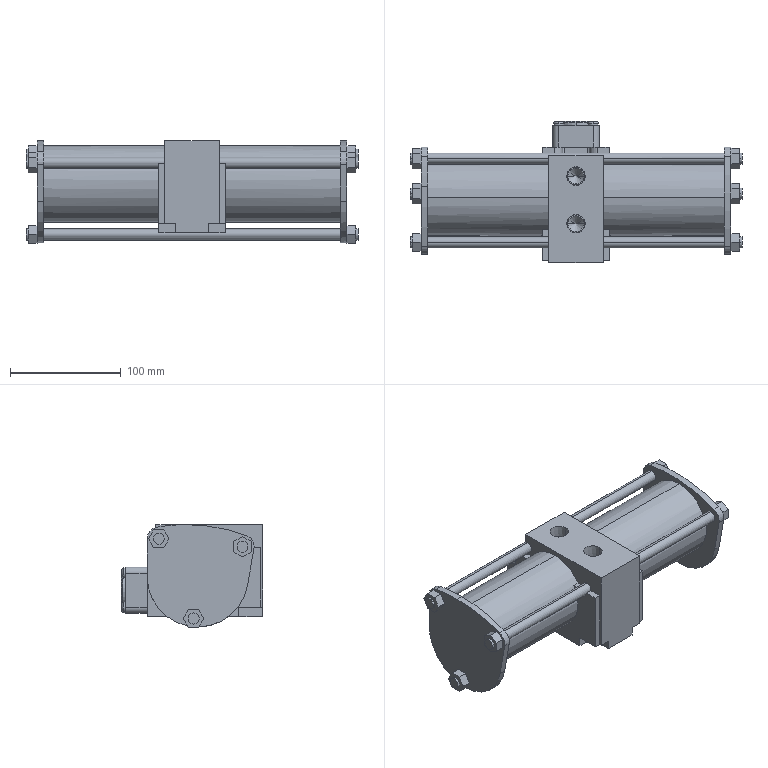Part | STEP file | VBA22A-03GN_VBA20A Body | 1 solid | 199 faces | box 300 x 127.5 x 92.8 mm | volume 1446394 mm3 | plane 100 | cylinder 65 | cone 26 | torus 8 | commonest cylinder face diameters 10 x21 9.5 x8 7.9 x6 14.3 x6 10.86 x4 21 x4